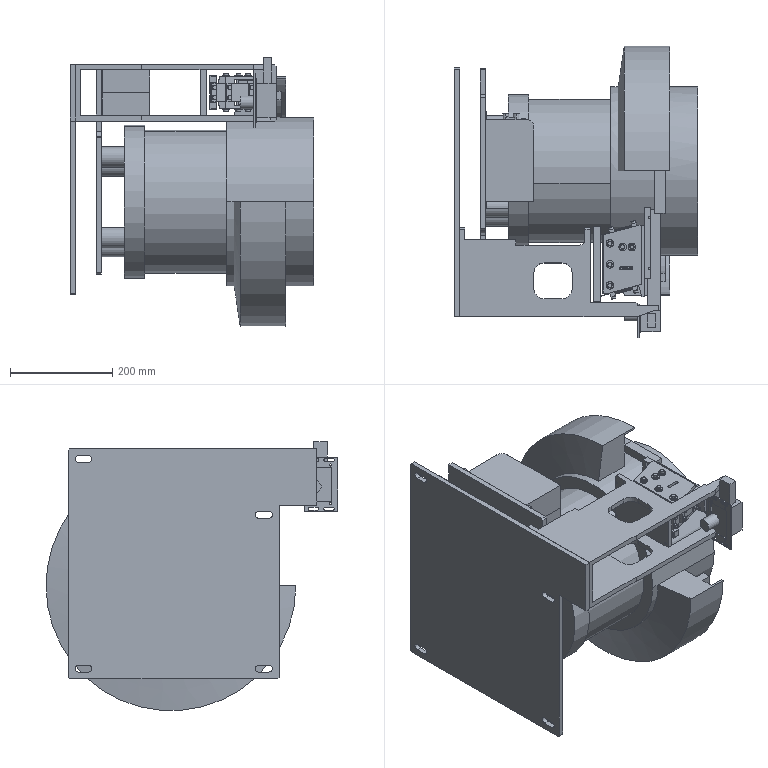Part | STEP file | COMPANY_C blow-air scheme, large part | 14 solids | 1108 faces | box 475 x 570.585 x 525.846 mm | volume 39693153 mm3 | plane 622 | cylinder 393 | torus 64 | other 20 | spline 8 | cone 1 | commonest cylinder face diameters 4.3 x66 8.5 x44 6 x35 5.3 x24 1.289 x20 1.524 x20